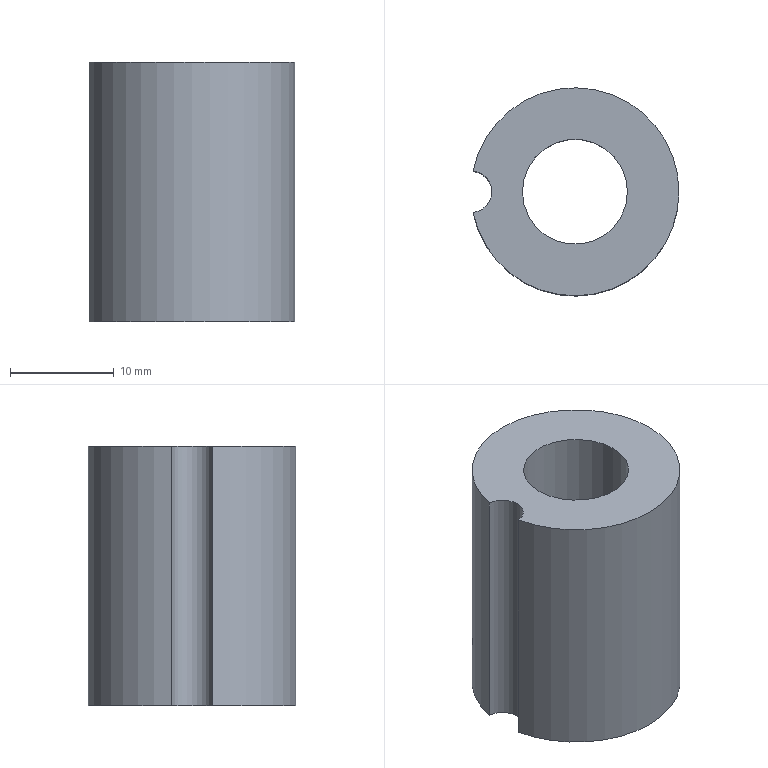Part | NX | features solid 2 | 1 solid | 7 faces | box 19.8 x 20 x 25 mm | volume 4943 mm3 | cylinder 4 | plane 3 | commonest cylinder face diameters 4 x1 10.1 x1 12.6 x1 20 x1
STEP:
#1=CARTESIAN_POINT('',(187.7,427.815,17.));
#2=VERTEX_POINT('',#1);
#3=CARTESIAN_POINT('',(187.7,427.815,42.));
#4=VERTEX_POINT('',#3);
#5=CARTESIAN_POINT('',(187.7,427.815,29.5));
#6=DIRECTION('',(0.,0.,1.));
#7=VECTOR('',#6,1000.);
#8=LINE('',#5,#7);
#9=EDGE_CURVE('',#2,#4,#8,.T.);
#10=ORIENTED_EDGE('',*,*,#9,.T.);
#11=CARTESIAN_POINT('',(187.7,423.835,42.));
#12=VERTEX_POINT('',#11);
#13=CARTESIAN_POINT('',(197.5,425.825,42.));
#14=DIRECTION('',(0.,0.,-1.));
#15=DIRECTION('',(-1.,0.,0.));
#16=AXIS2_PLACEMENT_3D('',#13,#14,#15);
#17=CIRCLE('',#16,10.);
#18=EDGE_CURVE('',#4,#12,#17,.T.);
#19=ORIENTED_EDGE('',*,*,#18,.T.);
#20=CARTESIAN_POINT('',(187.7,423.835,17.));
#21=VERTEX_POINT('',#20);
#22=CARTESIAN_POINT('',(187.7,423.835,29.5));
#23=DIRECTION('',(0.,0.,1.));
#24=VECTOR('',#23,1000.);
#25=LINE('',#22,#24);
#26=EDGE_CURVE('',#12,#21,#25,.F.);
#27=ORIENTED_EDGE('',*,*,#26,.T.);
#28=CARTESIAN_POINT('',(197.5,425.825,17.));
#29=DIRECTION('',(0.,0.,-1.));
#30=DIRECTION('',(-1.,0.,0.));
#31=AXIS2_PLACEMENT_3D('',#28,#29,#30);
#32=CIRCLE('',#31,10.);
#33=EDGE_CURVE('',#2,#21,#32,.T.);
#34=ORIENTED_EDGE('',*,*,#33,.F.);
#35=EDGE_LOOP('',(#10,#19,#27,#34));
#36=FACE_BOUND('',#35,.T.);
#37=CARTESIAN_POINT('',(197.5,425.825,17.));
#38=DIRECTION('',(0.,0.,1.));
#39=DIRECTION('',(-1.,0.,0.));
#40=AXIS2_PLACEMENT_3D('',#37,#38,#39);
#41=CYLINDRICAL_SURFACE('',#40,10.);
#42=ADVANCED_FACE('',(#36),#41,.T.);
#43=CARTESIAN_POINT('',(191.2,425.825,17.));
#44=VERTEX_POINT('',#43);
#45=CARTESIAN_POINT('',(197.5,425.825,17.));
#46=DIRECTION('',(0.,0.,-1.));
#47=DIRECTION('',(-1.,0.,0.));
#48=AXIS2_PLACEMENT_3D('',#45,#46,#47);
#49=CIRCLE('',#48,6.3);
#50=EDGE_CURVE('',#44,#44,#49,.T.);
#51=ORIENTED_EDGE('',*,*,#50,.F.);
#52=EDGE_LOOP('',(#51));
#53=FACE_BOUND('',#52,.T.);
#54=ORIENTED_EDGE('',*,*,#33,.T.);
#55=CARTESIAN_POINT('',(187.5,425.825,17.));
#56=DIRECTION('',(0.,0.,-1.));
#57=DIRECTION('',(-1.,0.,0.));
#58=AXIS2_PLACEMENT_3D('',#55,#56,#57);
#59=CIRCLE('',#58,2.);
#60=EDGE_CURVE('',#2,#21,#59,.T.);
#61=ORIENTED_EDGE('',*,*,#60,.F.);
#62=EDGE_LOOP('',(#54,#61));
#63=FACE_BOUND('',#62,.T.);
#64=CARTESIAN_POINT('',(197.5,425.825,17.));
#65=DIRECTION('',(0.,0.,1.));
#66=DIRECTION('',(-1.,0.,0.));
#67=AXIS2_PLACEMENT_3D('',#64,#65,#66);
#68=PLANE('',#67);
#69=ADVANCED_FACE('',(#53,#63),#68,.F.);
#70=CARTESIAN_POINT('',(192.45,425.825,42.));
#71=VERTEX_POINT('',#70);
#72=CARTESIAN_POINT('',(197.5,425.825,42.));
#73=DIRECTION('',(0.,0.,-1.));
#74=DIRECTION('',(-1.,0.,0.));
#75=AXIS2_PLACEMENT_3D('',#72,#73,#74);
#76=CIRCLE('',#75,5.05);
#77=EDGE_CURVE('',#71,#71,#76,.T.);
#78=ORIENTED_EDGE('',*,*,#77,.T.);
#79=EDGE_LOOP('',(#78));
#80=FACE_BOUND('',#79,.T.);
#81=CARTESIAN_POINT('',(187.5,425.825,42.));
#82=DIRECTION('',(0.,0.,-1.));
#83=DIRECTION('',(-1.,0.,0.));
#84=AXIS2_PLACEMENT_3D('',#81,#82,#83);
#85=CIRCLE('',#84,2.);
#86=EDGE_CURVE('',#4,#12,#85,.T.);
#87=ORIENTED_EDGE('',*,*,#86,.T.);
#88=ORIENTED_EDGE('',*,*,#18,.F.);
#89=EDGE_LOOP('',(#87,#88));
#90=FACE_BOUND('',#89,.T.);
#91=CARTESIAN_POINT('',(197.5,425.825,42.));
#92=DIRECTION('',(0.,0.,1.));
#93=DIRECTION('',(-1.,0.,0.));
#94=AXIS2_PLACEMENT_3D('',#91,#92,#93);
#95=PLANE('',#94);
#96=ADVANCED_FACE('',(#80,#90),#95,.T.);
#97=ORIENTED_EDGE('',*,*,#50,.T.);
#98=EDGE_LOOP('',(#97));
#99=FACE_BOUND('',#98,.T.);
#100=CARTESIAN_POINT('',(191.2,425.825,34.));
#101=VERTEX_POINT('',#100);
#102=CARTESIAN_POINT('',(197.5,425.825,34.));
#103=DIRECTION('',(0.,0.,-1.));
#104=DIRECTION('',(-1.,0.,0.));
#105=AXIS2_PLACEMENT_3D('',#102,#103,#104);
#106=CIRCLE('',#105,6.3);
#107=EDGE_CURVE('',#101,#101,#106,.T.);
#108=ORIENTED_EDGE('',*,*,#107,.F.);
#109=EDGE_LOOP('',(#108));
#110=FACE_BOUND('',#109,.T.);
#111=CARTESIAN_POINT('',(197.5,425.825,17.));
#112=DIRECTION('',(0.,0.,1.));
#113=DIRECTION('',(-1.,0.,0.));
#114=AXIS2_PLACEMENT_3D('',#111,#112,#113);
#115=CYLINDRICAL_SURFACE('',#114,6.3);
#116=ADVANCED_FACE('',(#99,#110),#115,.F.);
#117=CARTESIAN_POINT('',(192.45,425.825,34.));
#118=VERTEX_POINT('',#117);
#119=CARTESIAN_POINT('',(197.5,425.825,34.));
#120=DIRECTION('',(0.,0.,-1.));
#121=DIRECTION('',(-1.,0.,0.));
#122=AXIS2_PLACEMENT_3D('',#119,#120,#121);
#123=CIRCLE('',#122,5.05);
#124=EDGE_CURVE('',#118,#118,#123,.T.);
#125=ORIENTED_EDGE('',*,*,#124,.F.);
#126=EDGE_LOOP('',(#125));
#127=FACE_BOUND('',#126,.T.);
#128=ORIENTED_EDGE('',*,*,#107,.T.);
#129=EDGE_LOOP('',(#128));
#130=FACE_BOUND('',#129,.T.);
#131=CARTESIAN_POINT('',(197.5,425.825,34.));
#132=DIRECTION('',(0.,0.,1.));
#133=DIRECTION('',(-1.,0.,0.));
#134=AXIS2_PLACEMENT_3D('',#131,#132,#133);
#135=PLANE('',#134);
#136=ADVANCED_FACE('',(#127,#130),#135,.F.);
#137=ORIENTED_EDGE('',*,*,#9,.F.);
#138=ORIENTED_EDGE('',*,*,#60,.T.);
#139=ORIENTED_EDGE('',*,*,#26,.F.);
#140=ORIENTED_EDGE('',*,*,#86,.F.);
#141=EDGE_LOOP('',(#137,#138,#139,#140));
#142=FACE_BOUND('',#141,.T.);
#143=CARTESIAN_POINT('',(187.5,425.825,17.));
#144=DIRECTION('',(0.,0.,1.));
#145=DIRECTION('',(-1.,0.,0.));
#146=AXIS2_PLACEMENT_3D('',#143,#144,#145);
#147=CYLINDRICAL_SURFACE('',#146,2.);
#148=ADVANCED_FACE('',(#142),#147,.F.);
#149=ORIENTED_EDGE('',*,*,#77,.F.);
#150=EDGE_LOOP('',(#149));
#151=FACE_BOUND('',#150,.T.);
#152=ORIENTED_EDGE('',*,*,#124,.T.);
#153=EDGE_LOOP('',(#152));
#154=FACE_BOUND('',#153,.T.);
#155=CARTESIAN_POINT('',(197.5,425.825,17.));
#156=DIRECTION('',(0.,0.,1.));
#157=DIRECTION('',(-1.,0.,0.));
#158=AXIS2_PLACEMENT_3D('',#155,#156,#157);
#159=CYLINDRICAL_SURFACE('',#158,5.05);
#160=ADVANCED_FACE('',(#151,#154),#159,.F.);
#161=CLOSED_SHELL('',(#42,#69,#96,#116,#136,#148,#160));
#162=MANIFOLD_SOLID_BREP('',#161);
#163=(LENGTH_UNIT()NAMED_UNIT(*)SI_UNIT(.MILLI.,.METRE.));
#164=UNCERTAINTY_MEASURE_WITH_UNIT(LENGTH_MEASURE(0.00001),#163,'','');
#165=(NAMED_UNIT(*)PLANE_ANGLE_UNIT()SI_UNIT($,.RADIAN.));
#166=(NAMED_UNIT(*)SI_UNIT($,.STERADIAN.)SOLID_ANGLE_UNIT());
#167=(GEOMETRIC_REPRESENTATION_CONTEXT(3)GLOBAL_UNCERTAINTY_ASSIGNED_CONTEXT((#164))GLOBAL_UNIT_ASSIGNED_CONTEXT((#163,#165,#166))REPRESENTATION_CONTEXT('',''));
#168=ADVANCED_BREP_SHAPE_REPRESENTATION('',(#162),#167);